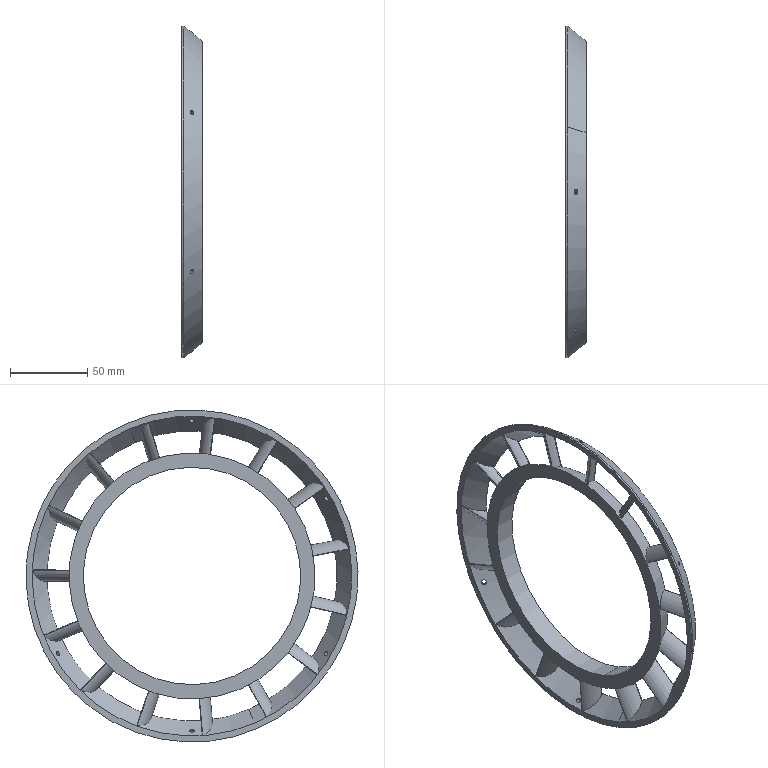Part | STEP file | Completa.sldasm-Part-58_Valor predeterminado | 1 solid | 99 faces | box 13.427 x 215.474 x 215.474 mm | volume 81310 mm3 | cylinder 89 | cone 6 | plane 4 | commonest cylinder face diameters 2 x30 0.4 x15 21.303 x15 35.24 x15 3.22 x10 141 x2